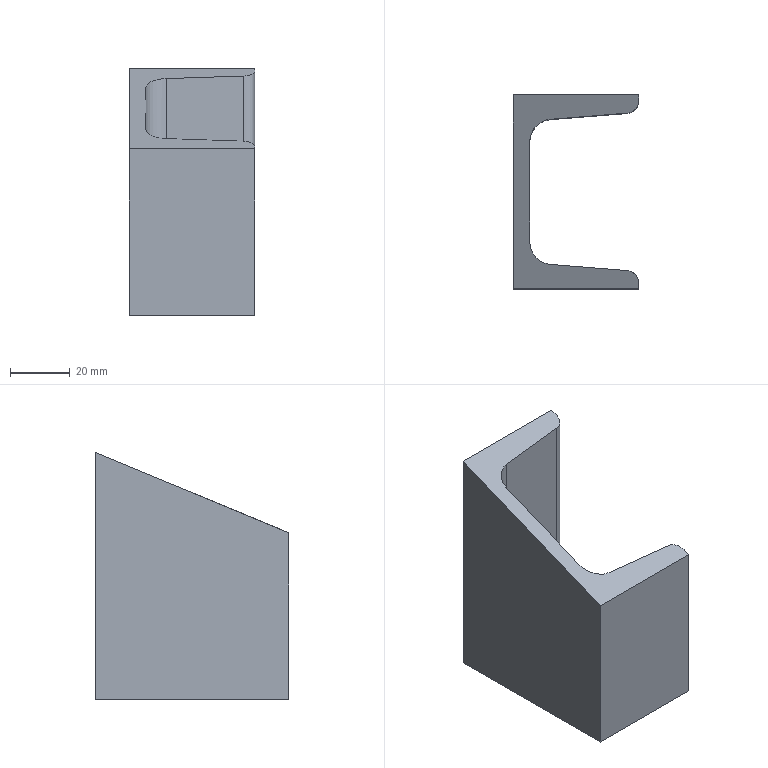Part | STEP file | DIN 1026-1 U 65 1785352380440 | 1 solid | 14 faces | box 42 x 65 x 82.843 mm | volume 62668 mm3 | plane 10 | cylinder 4 | commonest cylinder face diameters 8 x2 15 x2
STEP:
#1=CARTESIAN_POINT('',(5.5,-16.836,62.407));
#2=VERTEX_POINT('',#1);
#3=CARTESIAN_POINT('',(12.402,-24.312,59.31));
#4=VERTEX_POINT('',#3);
#5=CARTESIAN_POINT('',(13.,-16.836,62.407));
#6=DIRECTION('',(0.,-0.3827,0.9239));
#7=DIRECTION('',(0.,-0.9239,-0.3827));
#8=AXIS2_PLACEMENT_3D('',#5,#6,#7);
#9=ELLIPSE('',#8,8.118,7.5);
#10=EDGE_CURVE('',#2,#4,#9,.T.);
#11=ORIENTED_EDGE('',*,*,#10,.F.);
#12=CARTESIAN_POINT('',(5.5,16.836,76.354));
#13=VERTEX_POINT('',#12);
#14=CARTESIAN_POINT('',(5.5,-24.53,59.22));
#15=DIRECTION('',(0.,-0.9239,-0.3827));
#16=VECTOR('',#15,10.);
#17=LINE('',#14,#16);
#18=EDGE_CURVE('',#13,#2,#17,.T.);
#19=ORIENTED_EDGE('',*,*,#18,.F.);
#20=CARTESIAN_POINT('',(12.402,24.312,79.451));
#21=VERTEX_POINT('',#20);
#22=CARTESIAN_POINT('',(13.,16.836,76.354));
#23=DIRECTION('',(0.,-0.3827,0.9239));
#24=DIRECTION('',(0.,0.9239,0.3827));
#25=AXIS2_PLACEMENT_3D('',#22,#23,#24);
#26=ELLIPSE('',#25,8.118,7.5);
#27=EDGE_CURVE('',#21,#13,#26,.T.);
#28=ORIENTED_EDGE('',*,*,#27,.F.);
#29=CARTESIAN_POINT('',(38.319,26.386,80.31));
#30=VERTEX_POINT('',#29);
#31=CARTESIAN_POINT('',(15.613,24.569,79.558));
#32=DIRECTION('',(-0.9963,-0.0797,-0.03301));
#33=VECTOR('',#32,10.);
#34=LINE('',#31,#33);
#35=EDGE_CURVE('',#30,#21,#34,.T.);
#36=ORIENTED_EDGE('',*,*,#35,.F.);
#37=CARTESIAN_POINT('',(42.,30.373,81.962));
#38=VERTEX_POINT('',#37);
#39=CARTESIAN_POINT('',(38.,30.373,81.962));
#40=DIRECTION('',(0.,0.3827,-0.9239));
#41=DIRECTION('',(0.,0.9239,0.3827));
#42=AXIS2_PLACEMENT_3D('',#39,#40,#41);
#43=ELLIPSE('',#42,4.33,4.);
#44=EDGE_CURVE('',#38,#30,#43,.T.);
#45=ORIENTED_EDGE('',*,*,#44,.F.);
#46=CARTESIAN_POINT('',(42.,32.5,82.843));
#47=VERTEX_POINT('',#46);
#48=CARTESIAN_POINT('',(42.,-10.66,64.965));
#49=DIRECTION('',(0.,-0.9239,-0.3827));
#50=VECTOR('',#49,10.);
#51=LINE('',#48,#50);
#52=EDGE_CURVE('',#47,#38,#51,.T.);
#53=ORIENTED_EDGE('',*,*,#52,.F.);
#54=CARTESIAN_POINT('',(0.,32.5,82.843));
#55=VERTEX_POINT('',#54);
#56=CARTESIAN_POINT('',(10.5,32.5,82.843));
#57=DIRECTION('',(1.,0.,0.));
#58=VECTOR('',#57,10.);
#59=LINE('',#56,#58);
#60=EDGE_CURVE('',#55,#47,#59,.T.);
#61=ORIENTED_EDGE('',*,*,#60,.F.);
#62=CARTESIAN_POINT('',(0.,-32.5,55.919));
#63=VERTEX_POINT('',#62);
#64=CARTESIAN_POINT('',(0.,-24.53,59.22));
#65=DIRECTION('',(0.,0.9239,0.3827));
#66=VECTOR('',#65,10.);
#67=LINE('',#64,#66);
#68=EDGE_CURVE('',#63,#55,#67,.T.);
#69=ORIENTED_EDGE('',*,*,#68,.F.);
#70=CARTESIAN_POINT('',(42.,-32.5,55.919));
#71=VERTEX_POINT('',#70);
#72=CARTESIAN_POINT('',(21.,-32.5,55.919));
#73=DIRECTION('',(-1.,0.,0.));
#74=VECTOR('',#73,10.);
#75=LINE('',#72,#74);
#76=EDGE_CURVE('',#71,#63,#75,.T.);
#77=ORIENTED_EDGE('',*,*,#76,.F.);
#78=CARTESIAN_POINT('',(42.,-30.373,56.8));
#79=VERTEX_POINT('',#78);
#80=CARTESIAN_POINT('',(42.,-37.492,53.851));
#81=DIRECTION('',(0.,-0.9239,-0.3827));
#82=VECTOR('',#81,10.);
#83=LINE('',#80,#82);
#84=EDGE_CURVE('',#79,#71,#83,.T.);
#85=ORIENTED_EDGE('',*,*,#84,.F.);
#86=CARTESIAN_POINT('',(38.319,-26.386,58.452));
#87=VERTEX_POINT('',#86);
#88=CARTESIAN_POINT('',(38.,-30.373,56.8));
#89=DIRECTION('',(0.,0.3827,-0.9239));
#90=DIRECTION('',(0.,-0.9239,-0.3827));
#91=AXIS2_PLACEMENT_3D('',#88,#89,#90);
#92=ELLIPSE('',#91,4.33,4.);
#93=EDGE_CURVE('',#87,#79,#92,.T.);
#94=ORIENTED_EDGE('',*,*,#93,.F.);
#95=CARTESIAN_POINT('',(7.233,-23.899,59.482));
#96=DIRECTION('',(0.9963,-0.0797,-0.03301));
#97=VECTOR('',#96,10.);
#98=LINE('',#95,#97);
#99=EDGE_CURVE('',#4,#87,#98,.T.);
#100=ORIENTED_EDGE('',*,*,#99,.F.);
#101=EDGE_LOOP('',(#11,#19,#28,#36,#45,#53,#61,#69,#77,#85,#94,#100));
#102=FACE_OUTER_BOUND('',#101,.T.);
#103=CARTESIAN_POINT('',(0.,-24.53,59.22));
#104=DIRECTION('',(0.,0.3827,-0.9239));
#105=DIRECTION('',(-1.,0.,0.));
#106=AXIS2_PLACEMENT_3D('',#103,#104,#105);
#107=PLANE('',#106);
#108=ADVANCED_FACE('',(#102),#107,.F.);
#109=ORIENTED_EDGE('',*,*,#52,.T.);
#110=CARTESIAN_POINT('',(42.,30.373,0.));
#111=VERTEX_POINT('',#110);
#112=CARTESIAN_POINT('',(42.,30.373,0.));
#113=DIRECTION('',(0.,0.,1.));
#114=VECTOR('',#113,10.);
#115=LINE('',#112,#114);
#116=EDGE_CURVE('',#111,#38,#115,.T.);
#117=ORIENTED_EDGE('',*,*,#116,.F.);
#118=CARTESIAN_POINT('',(42.,32.5,0.));
#119=VERTEX_POINT('',#118);
#120=CARTESIAN_POINT('',(42.,16.25,0.));
#121=DIRECTION('',(0.,-1.,0.));
#122=VECTOR('',#121,10.);
#123=LINE('',#120,#122);
#124=EDGE_CURVE('',#119,#111,#123,.T.);
#125=ORIENTED_EDGE('',*,*,#124,.F.);
#126=CARTESIAN_POINT('',(42.,32.5,0.));
#127=DIRECTION('',(0.,0.,1.));
#128=VECTOR('',#127,10.);
#129=LINE('',#126,#128);
#130=EDGE_CURVE('',#119,#47,#129,.T.);
#131=ORIENTED_EDGE('',*,*,#130,.T.);
#132=EDGE_LOOP('',(#109,#117,#125,#131));
#133=FACE_OUTER_BOUND('',#132,.T.);
#134=CARTESIAN_POINT('',(42.,32.5,0.));
#135=DIRECTION('',(1.,0.,0.));
#136=DIRECTION('',(0.,0.,-1.));
#137=AXIS2_PLACEMENT_3D('',#134,#135,#136);
#138=PLANE('',#137);
#139=ADVANCED_FACE('',(#133),#138,.T.);
#140=ORIENTED_EDGE('',*,*,#44,.T.);
#141=CARTESIAN_POINT('',(38.319,26.386,0.));
#142=VERTEX_POINT('',#141);
#143=CARTESIAN_POINT('',(38.319,26.386,0.));
#144=DIRECTION('',(0.,0.,1.));
#145=VECTOR('',#144,10.);
#146=LINE('',#143,#145);
#147=EDGE_CURVE('',#142,#30,#146,.T.);
#148=ORIENTED_EDGE('',*,*,#147,.F.);
#149=CARTESIAN_POINT('',(38.,30.373,0.));
#150=DIRECTION('',(0.,0.,-1.));
#151=DIRECTION('',(-0.07975,0.9968,0.));
#152=AXIS2_PLACEMENT_3D('',#149,#150,#151);
#153=CIRCLE('',#152,4.);
#154=EDGE_CURVE('',#111,#142,#153,.T.);
#155=ORIENTED_EDGE('',*,*,#154,.F.);
#156=ORIENTED_EDGE('',*,*,#116,.T.);
#157=EDGE_LOOP('',(#140,#148,#155,#156));
#158=FACE_OUTER_BOUND('',#157,.T.);
#159=CARTESIAN_POINT('',(38.,30.373,0.));
#160=DIRECTION('',(0.,0.,1.));
#161=DIRECTION('',(-0.07975,0.9968,0.));
#162=AXIS2_PLACEMENT_3D('',#159,#160,#161);
#163=CYLINDRICAL_SURFACE('',#162,4.);
#164=ADVANCED_FACE('',(#158),#163,.T.);
#165=ORIENTED_EDGE('',*,*,#35,.T.);
#166=CARTESIAN_POINT('',(12.402,24.312,0.));
#167=VERTEX_POINT('',#166);
#168=CARTESIAN_POINT('',(12.402,24.312,0.));
#169=DIRECTION('',(0.,0.,1.));
#170=VECTOR('',#169,10.);
#171=LINE('',#168,#170);
#172=EDGE_CURVE('',#167,#21,#171,.T.);
#173=ORIENTED_EDGE('',*,*,#172,.F.);
#174=CARTESIAN_POINT('',(28.666,25.613,0.));
#175=DIRECTION('',(-0.9968,-0.07975,0.));
#176=VECTOR('',#175,10.);
#177=LINE('',#174,#176);
#178=EDGE_CURVE('',#142,#167,#177,.T.);
#179=ORIENTED_EDGE('',*,*,#178,.F.);
#180=ORIENTED_EDGE('',*,*,#147,.T.);
#181=EDGE_LOOP('',(#165,#173,#179,#180));
#182=FACE_OUTER_BOUND('',#181,.T.);
#183=CARTESIAN_POINT('',(38.319,26.386,0.));
#184=DIRECTION('',(0.07975,-0.9968,0.));
#185=DIRECTION('',(0.,0.,-1.));
#186=AXIS2_PLACEMENT_3D('',#183,#184,#185);
#187=PLANE('',#186);
#188=ADVANCED_FACE('',(#182),#187,.T.);
#189=ORIENTED_EDGE('',*,*,#27,.T.);
#190=CARTESIAN_POINT('',(5.5,16.836,0.));
#191=VERTEX_POINT('',#190);
#192=CARTESIAN_POINT('',(5.5,16.836,0.));
#193=DIRECTION('',(0.,0.,1.));
#194=VECTOR('',#193,10.);
#195=LINE('',#192,#194);
#196=EDGE_CURVE('',#191,#13,#195,.T.);
#197=ORIENTED_EDGE('',*,*,#196,.F.);
#198=CARTESIAN_POINT('',(13.,16.836,0.));
#199=DIRECTION('',(0.,0.,1.));
#200=DIRECTION('',(-0.07975,0.9968,0.));
#201=AXIS2_PLACEMENT_3D('',#198,#199,#200);
#202=CIRCLE('',#201,7.5);
#203=EDGE_CURVE('',#167,#191,#202,.T.);
#204=ORIENTED_EDGE('',*,*,#203,.F.);
#205=ORIENTED_EDGE('',*,*,#172,.T.);
#206=EDGE_LOOP('',(#189,#197,#204,#205));
#207=FACE_OUTER_BOUND('',#206,.T.);
#208=CARTESIAN_POINT('',(13.,16.836,0.));
#209=DIRECTION('',(0.,0.,1.));
#210=DIRECTION('',(-0.07975,0.9968,0.));
#211=AXIS2_PLACEMENT_3D('',#208,#209,#210);
#212=CYLINDRICAL_SURFACE('',#211,7.5);
#213=ADVANCED_FACE('',(#207),#212,.F.);
#214=ORIENTED_EDGE('',*,*,#18,.T.);
#215=CARTESIAN_POINT('',(5.5,-16.836,0.));
#216=VERTEX_POINT('',#215);
#217=CARTESIAN_POINT('',(5.5,-16.836,0.));
#218=DIRECTION('',(0.,0.,1.));
#219=VECTOR('',#218,10.);
#220=LINE('',#217,#219);
#221=EDGE_CURVE('',#216,#2,#220,.T.);
#222=ORIENTED_EDGE('',*,*,#221,.F.);
#223=CARTESIAN_POINT('',(5.5,0.,0.));
#224=DIRECTION('',(0.,-1.,0.));
#225=VECTOR('',#224,10.);
#226=LINE('',#223,#225);
#227=EDGE_CURVE('',#191,#216,#226,.T.);
#228=ORIENTED_EDGE('',*,*,#227,.F.);
#229=ORIENTED_EDGE('',*,*,#196,.T.);
#230=EDGE_LOOP('',(#214,#222,#228,#229));
#231=FACE_OUTER_BOUND('',#230,.T.);
#232=CARTESIAN_POINT('',(5.5,0.,0.));
#233=DIRECTION('',(1.,0.,0.));
#234=DIRECTION('',(0.,0.,-1.));
#235=AXIS2_PLACEMENT_3D('',#232,#233,#234);
#236=PLANE('',#235);
#237=ADVANCED_FACE('',(#231),#236,.T.);
#238=ORIENTED_EDGE('',*,*,#10,.T.);
#239=CARTESIAN_POINT('',(12.402,-24.312,0.));
#240=VERTEX_POINT('',#239);
#241=CARTESIAN_POINT('',(12.402,-24.312,0.));
#242=DIRECTION('',(0.,0.,1.));
#243=VECTOR('',#242,10.);
#244=LINE('',#241,#243);
#245=EDGE_CURVE('',#240,#4,#244,.T.);
#246=ORIENTED_EDGE('',*,*,#245,.F.);
#247=CARTESIAN_POINT('',(13.,-16.836,0.));
#248=DIRECTION('',(0.,0.,1.));
#249=DIRECTION('',(-1.,0.,0.));
#250=AXIS2_PLACEMENT_3D('',#247,#248,#249);
#251=CIRCLE('',#250,7.5);
#252=EDGE_CURVE('',#216,#240,#251,.T.);
#253=ORIENTED_EDGE('',*,*,#252,.F.);
#254=ORIENTED_EDGE('',*,*,#221,.T.);
#255=EDGE_LOOP('',(#238,#246,#253,#254));
#256=FACE_OUTER_BOUND('',#255,.T.);
#257=CARTESIAN_POINT('',(13.,-16.836,0.));
#258=DIRECTION('',(0.,0.,1.));
#259=DIRECTION('',(-1.,0.,0.));
#260=AXIS2_PLACEMENT_3D('',#257,#258,#259);
#261=CYLINDRICAL_SURFACE('',#260,7.5);
#262=ADVANCED_FACE('',(#256),#261,.F.);
#263=ORIENTED_EDGE('',*,*,#99,.T.);
#264=CARTESIAN_POINT('',(38.319,-26.386,0.));
#265=VERTEX_POINT('',#264);
#266=CARTESIAN_POINT('',(38.319,-26.386,0.));
#267=DIRECTION('',(0.,0.,1.));
#268=VECTOR('',#267,10.);
#269=LINE('',#266,#268);
#270=EDGE_CURVE('',#265,#87,#269,.T.);
#271=ORIENTED_EDGE('',*,*,#270,.F.);
#272=CARTESIAN_POINT('',(15.707,-24.577,0.));
#273=DIRECTION('',(0.9968,-0.07975,0.));
#274=VECTOR('',#273,10.);
#275=LINE('',#272,#274);
#276=EDGE_CURVE('',#240,#265,#275,.T.);
#277=ORIENTED_EDGE('',*,*,#276,.F.);
#278=ORIENTED_EDGE('',*,*,#245,.T.);
#279=EDGE_LOOP('',(#263,#271,#277,#278));
#280=FACE_OUTER_BOUND('',#279,.T.);
#281=CARTESIAN_POINT('',(12.402,-24.312,0.));
#282=DIRECTION('',(0.07975,0.9968,0.));
#283=DIRECTION('',(0.,0.,1.));
#284=AXIS2_PLACEMENT_3D('',#281,#282,#283);
#285=PLANE('',#284);
#286=ADVANCED_FACE('',(#280),#285,.T.);
#287=ORIENTED_EDGE('',*,*,#93,.T.);
#288=CARTESIAN_POINT('',(42.,-30.373,0.));
#289=VERTEX_POINT('',#288);
#290=CARTESIAN_POINT('',(42.,-30.373,0.));
#291=DIRECTION('',(0.,0.,1.));
#292=VECTOR('',#291,10.);
#293=LINE('',#290,#292);
#294=EDGE_CURVE('',#289,#79,#293,.T.);
#295=ORIENTED_EDGE('',*,*,#294,.F.);
#296=CARTESIAN_POINT('',(38.,-30.373,0.));
#297=DIRECTION('',(0.,0.,-1.));
#298=DIRECTION('',(-1.,0.,0.));
#299=AXIS2_PLACEMENT_3D('',#296,#297,#298);
#300=CIRCLE('',#299,4.);
#301=EDGE_CURVE('',#265,#289,#300,.T.);
#302=ORIENTED_EDGE('',*,*,#301,.F.);
#303=ORIENTED_EDGE('',*,*,#270,.T.);
#304=EDGE_LOOP('',(#287,#295,#302,#303));
#305=FACE_OUTER_BOUND('',#304,.T.);
#306=CARTESIAN_POINT('',(38.,-30.373,0.));
#307=DIRECTION('',(0.,0.,1.));
#308=DIRECTION('',(-1.,0.,0.));
#309=AXIS2_PLACEMENT_3D('',#306,#307,#308);
#310=CYLINDRICAL_SURFACE('',#309,4.);
#311=ADVANCED_FACE('',(#305),#310,.T.);
#312=ORIENTED_EDGE('',*,*,#84,.T.);
#313=CARTESIAN_POINT('',(42.,-32.5,0.));
#314=VERTEX_POINT('',#313);
#315=CARTESIAN_POINT('',(42.,-32.5,0.));
#316=DIRECTION('',(0.,0.,1.));
#317=VECTOR('',#316,10.);
#318=LINE('',#315,#317);
#319=EDGE_CURVE('',#314,#71,#318,.T.);
#320=ORIENTED_EDGE('',*,*,#319,.F.);
#321=CARTESIAN_POINT('',(42.,-15.186,0.));
#322=DIRECTION('',(0.,-1.,0.));
#323=VECTOR('',#322,10.);
#324=LINE('',#321,#323);
#325=EDGE_CURVE('',#289,#314,#324,.T.);
#326=ORIENTED_EDGE('',*,*,#325,.F.);
#327=ORIENTED_EDGE('',*,*,#294,.T.);
#328=EDGE_LOOP('',(#312,#320,#326,#327));
#329=FACE_OUTER_BOUND('',#328,.T.);
#330=CARTESIAN_POINT('',(42.,-30.373,0.));
#331=DIRECTION('',(1.,0.,0.));
#332=DIRECTION('',(0.,0.,-1.));
#333=AXIS2_PLACEMENT_3D('',#330,#331,#332);
#334=PLANE('',#333);
#335=ADVANCED_FACE('',(#329),#334,.T.);
#336=ORIENTED_EDGE('',*,*,#76,.T.);
#337=CARTESIAN_POINT('',(0.,-32.5,0.));
#338=VERTEX_POINT('',#337);
#339=CARTESIAN_POINT('',(0.,-32.5,0.));
#340=DIRECTION('',(0.,0.,1.));
#341=VECTOR('',#340,10.);
#342=LINE('',#339,#341);
#343=EDGE_CURVE('',#338,#63,#342,.T.);
#344=ORIENTED_EDGE('',*,*,#343,.F.);
#345=CARTESIAN_POINT('',(31.5,-32.5,0.));
#346=DIRECTION('',(-1.,0.,0.));
#347=VECTOR('',#346,10.);
#348=LINE('',#345,#347);
#349=EDGE_CURVE('',#314,#338,#348,.T.);
#350=ORIENTED_EDGE('',*,*,#349,.F.);
#351=ORIENTED_EDGE('',*,*,#319,.T.);
#352=EDGE_LOOP('',(#336,#344,#350,#351));
#353=FACE_OUTER_BOUND('',#352,.T.);
#354=CARTESIAN_POINT('',(42.,-32.5,0.));
#355=DIRECTION('',(0.,-1.,0.));
#356=DIRECTION('',(0.,0.,-1.));
#357=AXIS2_PLACEMENT_3D('',#354,#355,#356);
#358=PLANE('',#357);
#359=ADVANCED_FACE('',(#353),#358,.T.);
#360=ORIENTED_EDGE('',*,*,#68,.T.);
#361=CARTESIAN_POINT('',(0.,32.5,0.));
#362=VERTEX_POINT('',#361);
#363=CARTESIAN_POINT('',(0.,32.5,0.));
#364=DIRECTION('',(0.,0.,1.));
#365=VECTOR('',#364,10.);
#366=LINE('',#363,#365);
#367=EDGE_CURVE('',#362,#55,#366,.T.);
#368=ORIENTED_EDGE('',*,*,#367,.F.);
#369=CARTESIAN_POINT('',(0.,0.,0.));
#370=DIRECTION('',(0.,1.,0.));
#371=VECTOR('',#370,10.);
#372=LINE('',#369,#371);
#373=EDGE_CURVE('',#338,#362,#372,.T.);
#374=ORIENTED_EDGE('',*,*,#373,.F.);
#375=ORIENTED_EDGE('',*,*,#343,.T.);
#376=EDGE_LOOP('',(#360,#368,#374,#375));
#377=FACE_OUTER_BOUND('',#376,.T.);
#378=CARTESIAN_POINT('',(0.,0.,0.));
#379=DIRECTION('',(-1.,0.,0.));
#380=DIRECTION('',(0.,0.,1.));
#381=AXIS2_PLACEMENT_3D('',#378,#379,#380);
#382=PLANE('',#381);
#383=ADVANCED_FACE('',(#377),#382,.T.);
#384=ORIENTED_EDGE('',*,*,#60,.T.);
#385=ORIENTED_EDGE('',*,*,#130,.F.);
#386=CARTESIAN_POINT('',(10.5,32.5,0.));
#387=DIRECTION('',(1.,0.,0.));
#388=VECTOR('',#387,10.);
#389=LINE('',#386,#388);
#390=EDGE_CURVE('',#362,#119,#389,.T.);
#391=ORIENTED_EDGE('',*,*,#390,.F.);
#392=ORIENTED_EDGE('',*,*,#367,.T.);
#393=EDGE_LOOP('',(#384,#385,#391,#392));
#394=FACE_OUTER_BOUND('',#393,.T.);
#395=CARTESIAN_POINT('',(0.,32.5,0.));
#396=DIRECTION('',(0.,1.,0.));
#397=DIRECTION('',(0.,0.,1.));
#398=AXIS2_PLACEMENT_3D('',#395,#396,#397);
#399=PLANE('',#398);
#400=ADVANCED_FACE('',(#394),#399,.T.);
#401=ORIENTED_EDGE('',*,*,#390,.T.);
#402=ORIENTED_EDGE('',*,*,#124,.T.);
#403=ORIENTED_EDGE('',*,*,#154,.T.);
#404=ORIENTED_EDGE('',*,*,#178,.T.);
#405=ORIENTED_EDGE('',*,*,#203,.T.);
#406=ORIENTED_EDGE('',*,*,#227,.T.);
#407=ORIENTED_EDGE('',*,*,#252,.T.);
#408=ORIENTED_EDGE('',*,*,#276,.T.);
#409=ORIENTED_EDGE('',*,*,#301,.T.);
#410=ORIENTED_EDGE('',*,*,#325,.T.);
#411=ORIENTED_EDGE('',*,*,#349,.T.);
#412=ORIENTED_EDGE('',*,*,#373,.T.);
#413=EDGE_LOOP('',(#401,#402,#403,#404,#405,#406,#407,#408,#409,#410,#411,#412));
#414=FACE_OUTER_BOUND('',#413,.T.);
#415=CARTESIAN_POINT('',(21.,0.,0.));
#416=DIRECTION('',(0.,0.,1.));
#417=DIRECTION('',(1.,0.,0.));
#418=AXIS2_PLACEMENT_3D('',#415,#416,#417);
#419=PLANE('',#418);
#420=ADVANCED_FACE('',(#414),#419,.F.);
#421=CLOSED_SHELL('',(#108,#139,#164,#188,#213,#237,#262,#286,#311,#335,#359,#383,#400,#420));
#422=MANIFOLD_SOLID_BREP('',#421);
#423=(LENGTH_UNIT()NAMED_UNIT(*)SI_UNIT(.MILLI.,.METRE.));
#424=UNCERTAINTY_MEASURE_WITH_UNIT(LENGTH_MEASURE(0.01),#423,'','');
#425=(NAMED_UNIT(*)PLANE_ANGLE_UNIT()SI_UNIT($,.RADIAN.));
#426=(NAMED_UNIT(*)SI_UNIT($,.STERADIAN.)SOLID_ANGLE_UNIT());
#427=(GEOMETRIC_REPRESENTATION_CONTEXT(3)GLOBAL_UNCERTAINTY_ASSIGNED_CONTEXT((#424))GLOBAL_UNIT_ASSIGNED_CONTEXT((#423,#425,#426))REPRESENTATION_CONTEXT('',''));
#428=ADVANCED_BREP_SHAPE_REPRESENTATION('',(#422),#427);